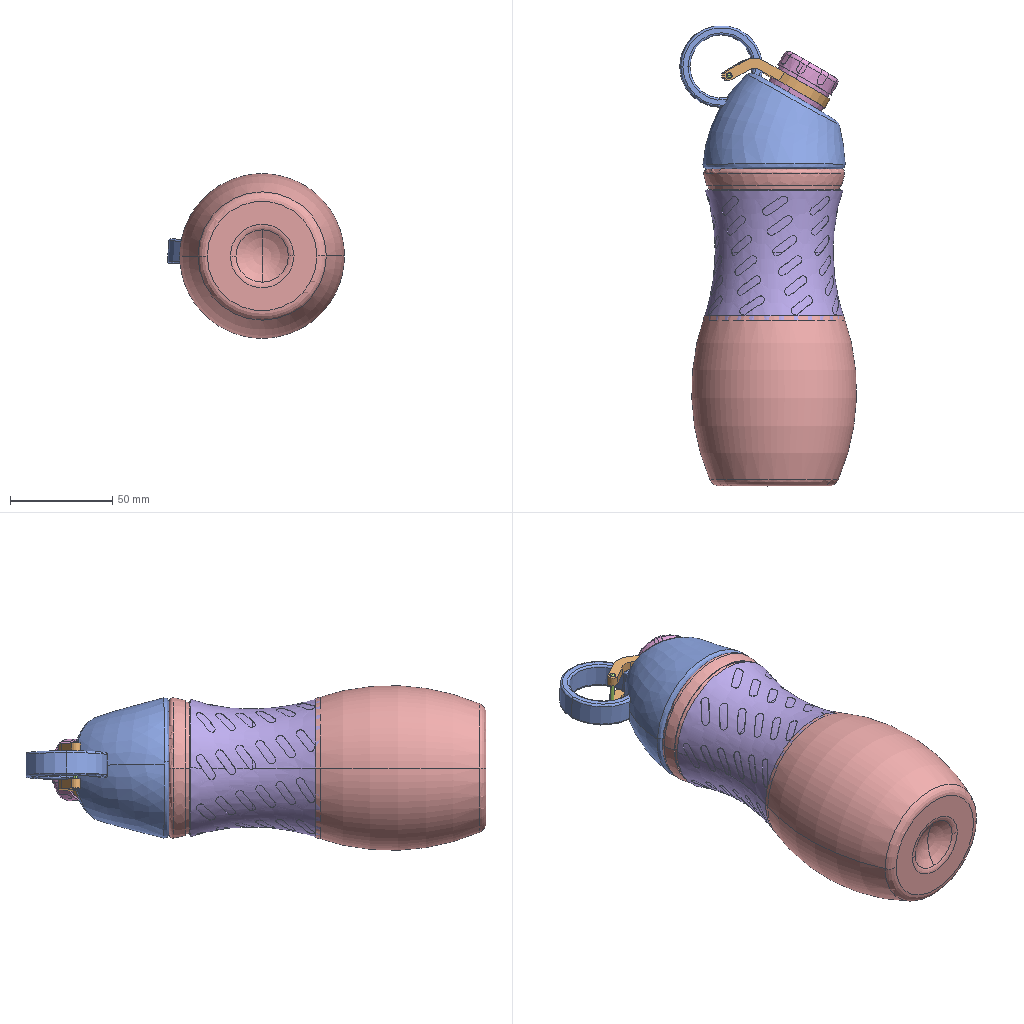Assembly | SolidWorks | 3 different items | 3 placed | box 86 x 225 x 80 mm
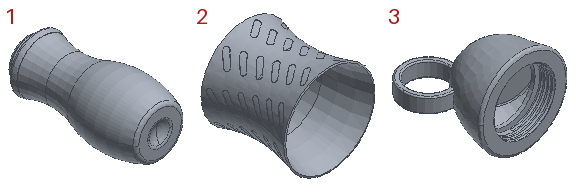Parts list (item | quantity | size | volume | features):
1 | x1 | - | 63029 mm3 | features ICE 3, BaseBody 2, Fillet 2, Blend 1, CombineBodies 1, DeleteBody 1, Helix 1, OffsetRefSurface 1, RevCut 1, Revolution 1, Sculpt 1, Shell 1, Sweep 1, Thicken 1
2 | x1 | 69.107 x 64.282 x 69.107 mm | 14161 mm3 | features BaseBody 2, DeleteBody 2, ICE 2, Blend 1, CirPattern 1, Emboss 1, Fillet 1, Helix 1, OffsetRefSurface 1, RefAxis 1, Revolution 1, Sculpt 1, Shell 1, Sweep 1, Thicken 1
3 | x1 | - | 42734 mm3 | features Fillet 6, ICE 6, Helix 3, Sculpt 3, BaseBody 2, DeleteBody 2, Shell 2, Sweep 2, Blend 1, CombineBodies 1, RefAxis 1, Revolution 1, Split 1, SweepCut 1
Mates (type | each side: item.copy, entity, surface, feature):
Concentric | 1.1 edge | 3.1 axis
Concentric | 1.1 edge | 2.1 edge
Coincident | 1.1 face plane Revolve1 | 3.1 face plane Loft1